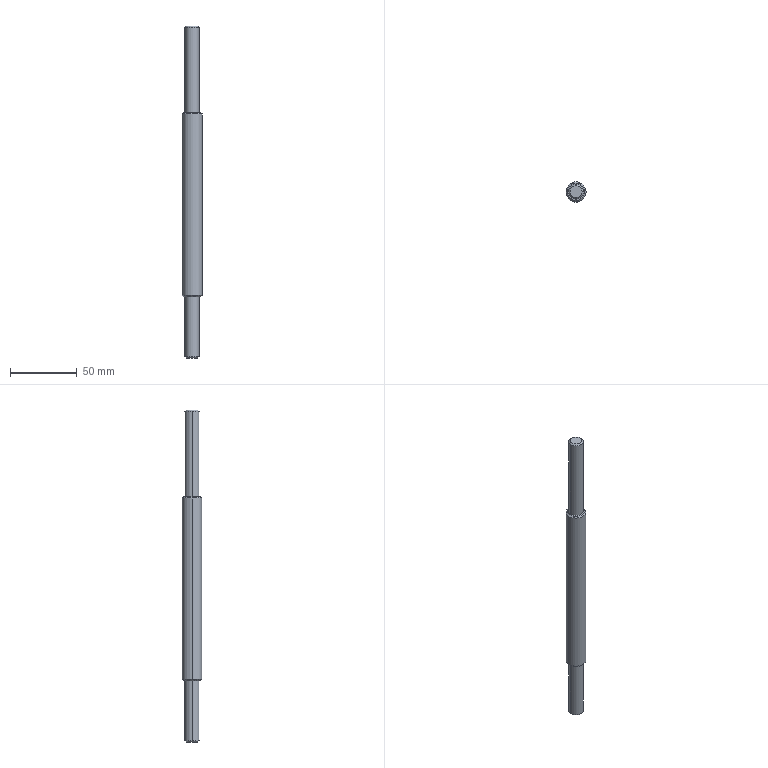Part | SolidWorks | features ICE 3, Chamfer 2, Extrusion 1 | 1 solid | 18 faces | box 15 x 15 x 249 mm | volume 34858 mm3 | cone 8 | cylinder 6 | plane 4 | commonest cylinder face diameters 11 x4 15 x2
STEP:
#1=CARTESIAN_POINT('',(-4.5,0.,-46.));
#2=VERTEX_POINT('',#1);
#3=CARTESIAN_POINT('',(4.5,0.,-46.));
#4=VERTEX_POINT('',#3);
#5=CARTESIAN_POINT('',(0.,0.,-46.));
#6=DIRECTION('',(0.,0.,-1.));
#7=DIRECTION('',(-1.,0.,0.));
#8=AXIS2_PLACEMENT_3D('',#5,#6,#7);
#9=CIRCLE('',#8,4.5);
#10=EDGE_CURVE('',#2,#4,#9,.T.);
#11=ORIENTED_EDGE('',*,*,#10,.F.);
#12=CARTESIAN_POINT('',(-5.5,0.,-45.));
#13=VERTEX_POINT('',#12);
#14=CARTESIAN_POINT('',(-4.5,0.,-46.));
#15=DIRECTION('',(-0.7071,0.,0.7071));
#16=VECTOR('',#15,1000.);
#17=LINE('',#14,#16);
#18=EDGE_CURVE('',#2,#13,#17,.T.);
#19=ORIENTED_EDGE('',*,*,#18,.T.);
#20=CARTESIAN_POINT('',(5.5,0.,-45.));
#21=VERTEX_POINT('',#20);
#22=CARTESIAN_POINT('',(0.,0.,-45.));
#23=DIRECTION('',(0.,0.,1.));
#24=DIRECTION('',(-1.,0.,0.));
#25=AXIS2_PLACEMENT_3D('',#22,#23,#24);
#26=CIRCLE('',#25,5.5);
#27=EDGE_CURVE('',#21,#13,#26,.T.);
#28=ORIENTED_EDGE('',*,*,#27,.F.);
#29=CARTESIAN_POINT('',(4.5,0.,-46.));
#30=DIRECTION('',(0.7071,0.,0.7071));
#31=VECTOR('',#30,1000.);
#32=LINE('',#29,#31);
#33=EDGE_CURVE('',#4,#21,#32,.T.);
#34=ORIENTED_EDGE('',*,*,#33,.F.);
#35=EDGE_LOOP('',(#11,#19,#28,#34));
#36=FACE_OUTER_BOUND('',#35,.T.);
#37=CARTESIAN_POINT('',(0.,0.,-46.));
#38=DIRECTION('',(0.,0.,1.));
#39=DIRECTION('',(1.,0.,0.));
#40=AXIS2_PLACEMENT_3D('',#37,#38,#39);
#41=CONICAL_SURFACE('',#40,4.5,0.7854);
#42=ADVANCED_FACE('',(#36),#41,.T.);
#43=ORIENTED_EDGE('',*,*,#27,.T.);
#44=CARTESIAN_POINT('',(-5.5,0.,0.));
#45=VERTEX_POINT('',#44);
#46=CARTESIAN_POINT('',(-5.5,0.,-46.));
#47=DIRECTION('',(0.,0.,1.));
#48=VECTOR('',#47,1000.);
#49=LINE('',#46,#48);
#50=EDGE_CURVE('',#13,#45,#49,.T.);
#51=ORIENTED_EDGE('',*,*,#50,.T.);
#52=CARTESIAN_POINT('',(5.5,0.,0.));
#53=VERTEX_POINT('',#52);
#54=CARTESIAN_POINT('',(0.,0.,0.));
#55=DIRECTION('',(0.,0.,-1.));
#56=DIRECTION('',(1.,0.,0.));
#57=AXIS2_PLACEMENT_3D('',#54,#55,#56);
#58=CIRCLE('',#57,5.5);
#59=EDGE_CURVE('',#45,#53,#58,.T.);
#60=ORIENTED_EDGE('',*,*,#59,.T.);
#61=CARTESIAN_POINT('',(5.5,0.,-46.));
#62=DIRECTION('',(0.,0.,1.));
#63=VECTOR('',#62,1000.);
#64=LINE('',#61,#63);
#65=EDGE_CURVE('',#21,#53,#64,.T.);
#66=ORIENTED_EDGE('',*,*,#65,.F.);
#67=EDGE_LOOP('',(#43,#51,#60,#66));
#68=FACE_OUTER_BOUND('',#67,.T.);
#69=CARTESIAN_POINT('',(0.,0.,-46.));
#70=DIRECTION('',(0.,0.,1.));
#71=DIRECTION('',(1.,0.,0.));
#72=AXIS2_PLACEMENT_3D('',#69,#70,#71);
#73=CYLINDRICAL_SURFACE('',#72,5.5);
#74=ADVANCED_FACE('',(#68),#73,.T.);
#75=CARTESIAN_POINT('',(6.5,0.,138.));
#76=VERTEX_POINT('',#75);
#77=CARTESIAN_POINT('',(-6.5,0.,138.));
#78=VERTEX_POINT('',#77);
#79=CARTESIAN_POINT('',(0.,0.,138.));
#80=DIRECTION('',(0.,0.,1.));
#81=DIRECTION('',(1.,0.,0.));
#82=AXIS2_PLACEMENT_3D('',#79,#80,#81);
#83=CIRCLE('',#82,6.5);
#84=EDGE_CURVE('',#76,#78,#83,.T.);
#85=ORIENTED_EDGE('',*,*,#84,.F.);
#86=CARTESIAN_POINT('',(7.5,0.,137.));
#87=VERTEX_POINT('',#86);
#88=CARTESIAN_POINT('',(6.5,0.,138.));
#89=DIRECTION('',(0.7071,0.,-0.7071));
#90=VECTOR('',#89,1000.);
#91=LINE('',#88,#90);
#92=EDGE_CURVE('',#76,#87,#91,.T.);
#93=ORIENTED_EDGE('',*,*,#92,.T.);
#94=CARTESIAN_POINT('',(-7.5,0.,137.));
#95=VERTEX_POINT('',#94);
#96=CARTESIAN_POINT('',(0.,0.,137.));
#97=DIRECTION('',(0.,0.,-1.));
#98=DIRECTION('',(1.,0.,0.));
#99=AXIS2_PLACEMENT_3D('',#96,#97,#98);
#100=CIRCLE('',#99,7.5);
#101=EDGE_CURVE('',#95,#87,#100,.T.);
#102=ORIENTED_EDGE('',*,*,#101,.F.);
#103=CARTESIAN_POINT('',(-6.5,0.,138.));
#104=DIRECTION('',(-0.7071,0.,-0.7071));
#105=VECTOR('',#104,1000.);
#106=LINE('',#103,#105);
#107=EDGE_CURVE('',#78,#95,#106,.T.);
#108=ORIENTED_EDGE('',*,*,#107,.F.);
#109=EDGE_LOOP('',(#85,#93,#102,#108));
#110=FACE_OUTER_BOUND('',#109,.T.);
#111=CARTESIAN_POINT('',(0.,0.,138.));
#112=DIRECTION('',(0.,0.,-1.));
#113=DIRECTION('',(-1.,0.,0.));
#114=AXIS2_PLACEMENT_3D('',#111,#112,#113);
#115=CONICAL_SURFACE('',#114,6.5,0.7854);
#116=ADVANCED_FACE('',(#110),#115,.T.);
#117=CARTESIAN_POINT('',(-6.5,0.,0.));
#118=VERTEX_POINT('',#117);
#119=CARTESIAN_POINT('',(6.5,0.,0.));
#120=VERTEX_POINT('',#119);
#121=CARTESIAN_POINT('',(0.,0.,0.));
#122=DIRECTION('',(0.,0.,-1.));
#123=DIRECTION('',(1.,0.,0.));
#124=AXIS2_PLACEMENT_3D('',#121,#122,#123);
#125=CIRCLE('',#124,6.5);
#126=EDGE_CURVE('',#118,#120,#125,.T.);
#127=ORIENTED_EDGE('',*,*,#126,.F.);
#128=CARTESIAN_POINT('',(-7.5,0.,1.));
#129=VERTEX_POINT('',#128);
#130=CARTESIAN_POINT('',(-7.5,0.,1.));
#131=DIRECTION('',(-0.7071,0.,0.7071));
#132=VECTOR('',#131,1000.);
#133=LINE('',#130,#132);
#134=EDGE_CURVE('',#118,#129,#133,.T.);
#135=ORIENTED_EDGE('',*,*,#134,.T.);
#136=CARTESIAN_POINT('',(7.5,0.,1.));
#137=VERTEX_POINT('',#136);
#138=CARTESIAN_POINT('',(0.,0.,1.));
#139=DIRECTION('',(0.,0.,1.));
#140=DIRECTION('',(1.,0.,0.));
#141=AXIS2_PLACEMENT_3D('',#138,#139,#140);
#142=CIRCLE('',#141,7.5);
#143=EDGE_CURVE('',#137,#129,#142,.T.);
#144=ORIENTED_EDGE('',*,*,#143,.F.);
#145=CARTESIAN_POINT('',(7.5,0.,1.));
#146=DIRECTION('',(0.7071,0.,0.7071));
#147=VECTOR('',#146,1000.);
#148=LINE('',#145,#147);
#149=EDGE_CURVE('',#120,#137,#148,.T.);
#150=ORIENTED_EDGE('',*,*,#149,.F.);
#151=EDGE_LOOP('',(#127,#135,#144,#150));
#152=FACE_OUTER_BOUND('',#151,.T.);
#153=CARTESIAN_POINT('',(0.,0.,1.));
#154=DIRECTION('',(0.,0.,1.));
#155=DIRECTION('',(1.,0.,0.));
#156=AXIS2_PLACEMENT_3D('',#153,#154,#155);
#157=CONICAL_SURFACE('',#156,7.5,0.7854);
#158=ADVANCED_FACE('',(#152),#157,.T.);
#159=CARTESIAN_POINT('',(4.5,0.,203.));
#160=VERTEX_POINT('',#159);
#161=CARTESIAN_POINT('',(-4.5,0.,203.));
#162=VERTEX_POINT('',#161);
#163=CARTESIAN_POINT('',(0.,0.,203.));
#164=DIRECTION('',(0.,0.,1.));
#165=DIRECTION('',(1.,0.,0.));
#166=AXIS2_PLACEMENT_3D('',#163,#164,#165);
#167=CIRCLE('',#166,4.5);
#168=EDGE_CURVE('',#160,#162,#167,.T.);
#169=ORIENTED_EDGE('',*,*,#168,.F.);
#170=CARTESIAN_POINT('',(5.5,0.,202.));
#171=VERTEX_POINT('',#170);
#172=CARTESIAN_POINT('',(4.5,0.,203.));
#173=DIRECTION('',(0.7071,0.,-0.7071));
#174=VECTOR('',#173,1000.);
#175=LINE('',#172,#174);
#176=EDGE_CURVE('',#160,#171,#175,.T.);
#177=ORIENTED_EDGE('',*,*,#176,.T.);
#178=CARTESIAN_POINT('',(-5.5,0.,202.));
#179=VERTEX_POINT('',#178);
#180=CARTESIAN_POINT('',(0.,0.,202.));
#181=DIRECTION('',(0.,0.,-1.));
#182=DIRECTION('',(1.,0.,0.));
#183=AXIS2_PLACEMENT_3D('',#180,#181,#182);
#184=CIRCLE('',#183,5.5);
#185=EDGE_CURVE('',#179,#171,#184,.T.);
#186=ORIENTED_EDGE('',*,*,#185,.F.);
#187=CARTESIAN_POINT('',(-4.5,0.,203.));
#188=DIRECTION('',(-0.7071,0.,-0.7071));
#189=VECTOR('',#188,1000.);
#190=LINE('',#187,#189);
#191=EDGE_CURVE('',#162,#179,#190,.T.);
#192=ORIENTED_EDGE('',*,*,#191,.F.);
#193=EDGE_LOOP('',(#169,#177,#186,#192));
#194=FACE_OUTER_BOUND('',#193,.T.);
#195=CARTESIAN_POINT('',(0.,0.,203.));
#196=DIRECTION('',(0.,0.,-1.));
#197=DIRECTION('',(-1.,0.,0.));
#198=AXIS2_PLACEMENT_3D('',#195,#196,#197);
#199=CONICAL_SURFACE('',#198,4.5,0.7854);
#200=ADVANCED_FACE('',(#194),#199,.T.);
#201=ORIENTED_EDGE('',*,*,#185,.T.);
#202=CARTESIAN_POINT('',(5.5,0.,138.));
#203=VERTEX_POINT('',#202);
#204=CARTESIAN_POINT('',(5.5,0.,158.));
#205=DIRECTION('',(0.,0.,-1.));
#206=VECTOR('',#205,1000.);
#207=LINE('',#204,#206);
#208=EDGE_CURVE('',#171,#203,#207,.T.);
#209=ORIENTED_EDGE('',*,*,#208,.T.);
#210=CARTESIAN_POINT('',(-5.5,0.,138.));
#211=VERTEX_POINT('',#210);
#212=CARTESIAN_POINT('',(0.,0.,138.));
#213=DIRECTION('',(0.,0.,1.));
#214=DIRECTION('',(1.,0.,0.));
#215=AXIS2_PLACEMENT_3D('',#212,#213,#214);
#216=CIRCLE('',#215,5.5);
#217=EDGE_CURVE('',#203,#211,#216,.T.);
#218=ORIENTED_EDGE('',*,*,#217,.T.);
#219=CARTESIAN_POINT('',(-5.5,0.,158.));
#220=DIRECTION('',(0.,0.,-1.));
#221=VECTOR('',#220,1000.);
#222=LINE('',#219,#221);
#223=EDGE_CURVE('',#179,#211,#222,.T.);
#224=ORIENTED_EDGE('',*,*,#223,.F.);
#225=EDGE_LOOP('',(#201,#209,#218,#224));
#226=FACE_OUTER_BOUND('',#225,.T.);
#227=CARTESIAN_POINT('',(0.,0.,158.));
#228=DIRECTION('',(0.,0.,-1.));
#229=DIRECTION('',(-1.,0.,0.));
#230=AXIS2_PLACEMENT_3D('',#227,#228,#229);
#231=CYLINDRICAL_SURFACE('',#230,5.5);
#232=ADVANCED_FACE('',(#226),#231,.T.);
#233=ORIENTED_EDGE('',*,*,#101,.T.);
#234=CARTESIAN_POINT('',(7.5,0.,138.));
#235=DIRECTION('',(0.,0.,-1.));
#236=VECTOR('',#235,1000.);
#237=LINE('',#234,#236);
#238=EDGE_CURVE('',#87,#137,#237,.T.);
#239=ORIENTED_EDGE('',*,*,#238,.T.);
#240=ORIENTED_EDGE('',*,*,#143,.T.);
#241=CARTESIAN_POINT('',(-7.5,0.,138.));
#242=DIRECTION('',(0.,0.,-1.));
#243=VECTOR('',#242,1000.);
#244=LINE('',#241,#243);
#245=EDGE_CURVE('',#95,#129,#244,.T.);
#246=ORIENTED_EDGE('',*,*,#245,.F.);
#247=EDGE_LOOP('',(#233,#239,#240,#246));
#248=FACE_OUTER_BOUND('',#247,.T.);
#249=CARTESIAN_POINT('',(0.,0.,138.));
#250=DIRECTION('',(0.,0.,-1.));
#251=DIRECTION('',(-1.,0.,0.));
#252=AXIS2_PLACEMENT_3D('',#249,#250,#251);
#253=CYLINDRICAL_SURFACE('',#252,7.5);
#254=ADVANCED_FACE('',(#248),#253,.T.);
#255=CARTESIAN_POINT('',(0.,0.,0.));
#256=DIRECTION('',(0.,0.,-1.));
#257=DIRECTION('',(1.,0.,0.));
#258=AXIS2_PLACEMENT_3D('',#255,#256,#257);
#259=CIRCLE('',#258,6.5);
#260=EDGE_CURVE('',#120,#118,#259,.T.);
#261=ORIENTED_EDGE('',*,*,#260,.T.);
#262=ORIENTED_EDGE('',*,*,#126,.T.);
#263=EDGE_LOOP('',(#261,#262));
#264=FACE_OUTER_BOUND('',#263,.T.);
#265=CARTESIAN_POINT('',(0.,0.,0.));
#266=DIRECTION('',(0.,0.,-1.));
#267=DIRECTION('',(1.,0.,0.));
#268=AXIS2_PLACEMENT_3D('',#265,#266,#267);
#269=CIRCLE('',#268,5.5);
#270=EDGE_CURVE('',#53,#45,#269,.T.);
#271=ORIENTED_EDGE('',*,*,#270,.F.);
#272=ORIENTED_EDGE('',*,*,#59,.F.);
#273=EDGE_LOOP('',(#271,#272));
#274=FACE_BOUND('',#273,.T.);
#275=CARTESIAN_POINT('',(0.,0.,0.));
#276=DIRECTION('',(0.,0.,1.));
#277=DIRECTION('',(1.,0.,0.));
#278=AXIS2_PLACEMENT_3D('',#275,#276,#277);
#279=PLANE('',#278);
#280=ADVANCED_FACE('',(#264,#274),#279,.F.);
#281=CARTESIAN_POINT('',(0.,0.,138.));
#282=DIRECTION('',(0.,0.,1.));
#283=DIRECTION('',(1.,0.,0.));
#284=AXIS2_PLACEMENT_3D('',#281,#282,#283);
#285=CIRCLE('',#284,6.5);
#286=EDGE_CURVE('',#78,#76,#285,.T.);
#287=ORIENTED_EDGE('',*,*,#286,.T.);
#288=ORIENTED_EDGE('',*,*,#84,.T.);
#289=EDGE_LOOP('',(#287,#288));
#290=FACE_OUTER_BOUND('',#289,.T.);
#291=CARTESIAN_POINT('',(0.,0.,138.));
#292=DIRECTION('',(0.,0.,1.));
#293=DIRECTION('',(1.,0.,0.));
#294=AXIS2_PLACEMENT_3D('',#291,#292,#293);
#295=CIRCLE('',#294,5.5);
#296=EDGE_CURVE('',#211,#203,#295,.T.);
#297=ORIENTED_EDGE('',*,*,#296,.F.);
#298=ORIENTED_EDGE('',*,*,#217,.F.);
#299=EDGE_LOOP('',(#297,#298));
#300=FACE_BOUND('',#299,.T.);
#301=CARTESIAN_POINT('',(0.,0.,138.));
#302=DIRECTION('',(0.,0.,1.));
#303=DIRECTION('',(1.,0.,0.));
#304=AXIS2_PLACEMENT_3D('',#301,#302,#303);
#305=PLANE('',#304);
#306=ADVANCED_FACE('',(#290,#300),#305,.T.);
#307=ORIENTED_EDGE('',*,*,#238,.F.);
#308=CARTESIAN_POINT('',(0.,0.,137.));
#309=DIRECTION('',(0.,0.,-1.));
#310=DIRECTION('',(1.,0.,0.));
#311=AXIS2_PLACEMENT_3D('',#308,#309,#310);
#312=CIRCLE('',#311,7.5);
#313=EDGE_CURVE('',#87,#95,#312,.T.);
#314=ORIENTED_EDGE('',*,*,#313,.T.);
#315=ORIENTED_EDGE('',*,*,#245,.T.);
#316=CARTESIAN_POINT('',(0.,0.,1.));
#317=DIRECTION('',(0.,0.,1.));
#318=DIRECTION('',(1.,0.,0.));
#319=AXIS2_PLACEMENT_3D('',#316,#317,#318);
#320=CIRCLE('',#319,7.5);
#321=EDGE_CURVE('',#129,#137,#320,.T.);
#322=ORIENTED_EDGE('',*,*,#321,.T.);
#323=EDGE_LOOP('',(#307,#314,#315,#322));
#324=FACE_OUTER_BOUND('',#323,.T.);
#325=CARTESIAN_POINT('',(0.,0.,138.));
#326=DIRECTION('',(0.,0.,-1.));
#327=DIRECTION('',(-1.,0.,0.));
#328=AXIS2_PLACEMENT_3D('',#325,#326,#327);
#329=CYLINDRICAL_SURFACE('',#328,7.5);
#330=ADVANCED_FACE('',(#324),#329,.T.);
#331=ORIENTED_EDGE('',*,*,#208,.F.);
#332=CARTESIAN_POINT('',(0.,0.,202.));
#333=DIRECTION('',(0.,0.,-1.));
#334=DIRECTION('',(1.,0.,0.));
#335=AXIS2_PLACEMENT_3D('',#332,#333,#334);
#336=CIRCLE('',#335,5.5);
#337=EDGE_CURVE('',#171,#179,#336,.T.);
#338=ORIENTED_EDGE('',*,*,#337,.T.);
#339=ORIENTED_EDGE('',*,*,#223,.T.);
#340=ORIENTED_EDGE('',*,*,#296,.T.);
#341=EDGE_LOOP('',(#331,#338,#339,#340));
#342=FACE_OUTER_BOUND('',#341,.T.);
#343=CARTESIAN_POINT('',(0.,0.,158.));
#344=DIRECTION('',(0.,0.,-1.));
#345=DIRECTION('',(-1.,0.,0.));
#346=AXIS2_PLACEMENT_3D('',#343,#344,#345);
#347=CYLINDRICAL_SURFACE('',#346,5.5);
#348=ADVANCED_FACE('',(#342),#347,.T.);
#349=CARTESIAN_POINT('',(0.,0.,203.));
#350=DIRECTION('',(0.,0.,1.));
#351=DIRECTION('',(1.,0.,0.));
#352=AXIS2_PLACEMENT_3D('',#349,#350,#351);
#353=CIRCLE('',#352,4.5);
#354=EDGE_CURVE('',#162,#160,#353,.T.);
#355=ORIENTED_EDGE('',*,*,#354,.T.);
#356=ORIENTED_EDGE('',*,*,#168,.T.);
#357=EDGE_LOOP('',(#355,#356));
#358=FACE_OUTER_BOUND('',#357,.T.);
#359=CARTESIAN_POINT('',(0.,0.,203.));
#360=DIRECTION('',(0.,0.,1.));
#361=DIRECTION('',(1.,0.,0.));
#362=AXIS2_PLACEMENT_3D('',#359,#360,#361);
#363=PLANE('',#362);
#364=ADVANCED_FACE('',(#358),#363,.T.);
#365=ORIENTED_EDGE('',*,*,#176,.F.);
#366=ORIENTED_EDGE('',*,*,#354,.F.);
#367=ORIENTED_EDGE('',*,*,#191,.T.);
#368=ORIENTED_EDGE('',*,*,#337,.F.);
#369=EDGE_LOOP('',(#365,#366,#367,#368));
#370=FACE_OUTER_BOUND('',#369,.T.);
#371=CARTESIAN_POINT('',(0.,0.,203.));
#372=DIRECTION('',(0.,0.,-1.));
#373=DIRECTION('',(-1.,0.,0.));
#374=AXIS2_PLACEMENT_3D('',#371,#372,#373);
#375=CONICAL_SURFACE('',#374,4.5,0.7854);
#376=ADVANCED_FACE('',(#370),#375,.T.);
#377=ORIENTED_EDGE('',*,*,#134,.F.);
#378=ORIENTED_EDGE('',*,*,#260,.F.);
#379=ORIENTED_EDGE('',*,*,#149,.T.);
#380=ORIENTED_EDGE('',*,*,#321,.F.);
#381=EDGE_LOOP('',(#377,#378,#379,#380));
#382=FACE_OUTER_BOUND('',#381,.T.);
#383=CARTESIAN_POINT('',(0.,0.,1.));
#384=DIRECTION('',(0.,0.,1.));
#385=DIRECTION('',(1.,0.,0.));
#386=AXIS2_PLACEMENT_3D('',#383,#384,#385);
#387=CONICAL_SURFACE('',#386,7.5,0.7854);
#388=ADVANCED_FACE('',(#382),#387,.T.);
#389=ORIENTED_EDGE('',*,*,#92,.F.);
#390=ORIENTED_EDGE('',*,*,#286,.F.);
#391=ORIENTED_EDGE('',*,*,#107,.T.);
#392=ORIENTED_EDGE('',*,*,#313,.F.);
#393=EDGE_LOOP('',(#389,#390,#391,#392));
#394=FACE_OUTER_BOUND('',#393,.T.);
#395=CARTESIAN_POINT('',(0.,0.,138.));
#396=DIRECTION('',(0.,0.,-1.));
#397=DIRECTION('',(-1.,0.,0.));
#398=AXIS2_PLACEMENT_3D('',#395,#396,#397);
#399=CONICAL_SURFACE('',#398,6.5,0.7854);
#400=ADVANCED_FACE('',(#394),#399,.T.);
#401=ORIENTED_EDGE('',*,*,#50,.F.);
#402=CARTESIAN_POINT('',(0.,0.,-45.));
#403=DIRECTION('',(0.,0.,1.));
#404=DIRECTION('',(-1.,0.,0.));
#405=AXIS2_PLACEMENT_3D('',#402,#403,#404);
#406=CIRCLE('',#405,5.5);
#407=EDGE_CURVE('',#13,#21,#406,.T.);
#408=ORIENTED_EDGE('',*,*,#407,.T.);
#409=ORIENTED_EDGE('',*,*,#65,.T.);
#410=ORIENTED_EDGE('',*,*,#270,.T.);
#411=EDGE_LOOP('',(#401,#408,#409,#410));
#412=FACE_OUTER_BOUND('',#411,.T.);
#413=CARTESIAN_POINT('',(0.,0.,-46.));
#414=DIRECTION('',(0.,0.,1.));
#415=DIRECTION('',(1.,0.,0.));
#416=AXIS2_PLACEMENT_3D('',#413,#414,#415);
#417=CYLINDRICAL_SURFACE('',#416,5.5);
#418=ADVANCED_FACE('',(#412),#417,.T.);
#419=CARTESIAN_POINT('',(0.,0.,-46.));
#420=DIRECTION('',(0.,0.,-1.));
#421=DIRECTION('',(-1.,0.,0.));
#422=AXIS2_PLACEMENT_3D('',#419,#420,#421);
#423=CIRCLE('',#422,4.5);
#424=EDGE_CURVE('',#4,#2,#423,.T.);
#425=ORIENTED_EDGE('',*,*,#424,.T.);
#426=ORIENTED_EDGE('',*,*,#10,.T.);
#427=EDGE_LOOP('',(#425,#426));
#428=FACE_OUTER_BOUND('',#427,.T.);
#429=CARTESIAN_POINT('',(0.,0.,-46.));
#430=DIRECTION('',(0.,0.,-1.));
#431=DIRECTION('',(-1.,0.,0.));
#432=AXIS2_PLACEMENT_3D('',#429,#430,#431);
#433=PLANE('',#432);
#434=ADVANCED_FACE('',(#428),#433,.T.);
#435=ORIENTED_EDGE('',*,*,#18,.F.);
#436=ORIENTED_EDGE('',*,*,#424,.F.);
#437=ORIENTED_EDGE('',*,*,#33,.T.);
#438=ORIENTED_EDGE('',*,*,#407,.F.);
#439=EDGE_LOOP('',(#435,#436,#437,#438));
#440=FACE_OUTER_BOUND('',#439,.T.);
#441=CARTESIAN_POINT('',(0.,0.,-46.));
#442=DIRECTION('',(0.,0.,1.));
#443=DIRECTION('',(1.,0.,0.));
#444=AXIS2_PLACEMENT_3D('',#441,#442,#443);
#445=CONICAL_SURFACE('',#444,4.5,0.7854);
#446=ADVANCED_FACE('',(#440),#445,.T.);
#447=CLOSED_SHELL('',(#42,#74,#116,#158,#200,#232,#254,#280,#306,#330,#348,#364,#376,#388,#400,#418,#434,#446));
#448=MANIFOLD_SOLID_BREP('',#447);
#449=CARTESIAN_POINT('',(0.,0.,0.));
#450=DIRECTION('',(0.,0.,1.));
#451=DIRECTION('',(1.,0.,0.));
#452=AXIS2_PLACEMENT_3D('',#449,#450,#451);
#453=(LENGTH_UNIT()NAMED_UNIT(*)SI_UNIT(.MILLI.,.METRE.));
#454=UNCERTAINTY_MEASURE_WITH_UNIT(LENGTH_MEASURE(0.00001),#453,'','');
#455=(NAMED_UNIT(*)PLANE_ANGLE_UNIT()SI_UNIT($,.RADIAN.));
#456=(NAMED_UNIT(*)SI_UNIT($,.STERADIAN.)SOLID_ANGLE_UNIT());
#457=(GEOMETRIC_REPRESENTATION_CONTEXT(3)GLOBAL_UNCERTAINTY_ASSIGNED_CONTEXT((#454))GLOBAL_UNIT_ASSIGNED_CONTEXT((#453,#455,#456))REPRESENTATION_CONTEXT('',''));
#458=ADVANCED_BREP_SHAPE_REPRESENTATION('',(#448,#452),#457);